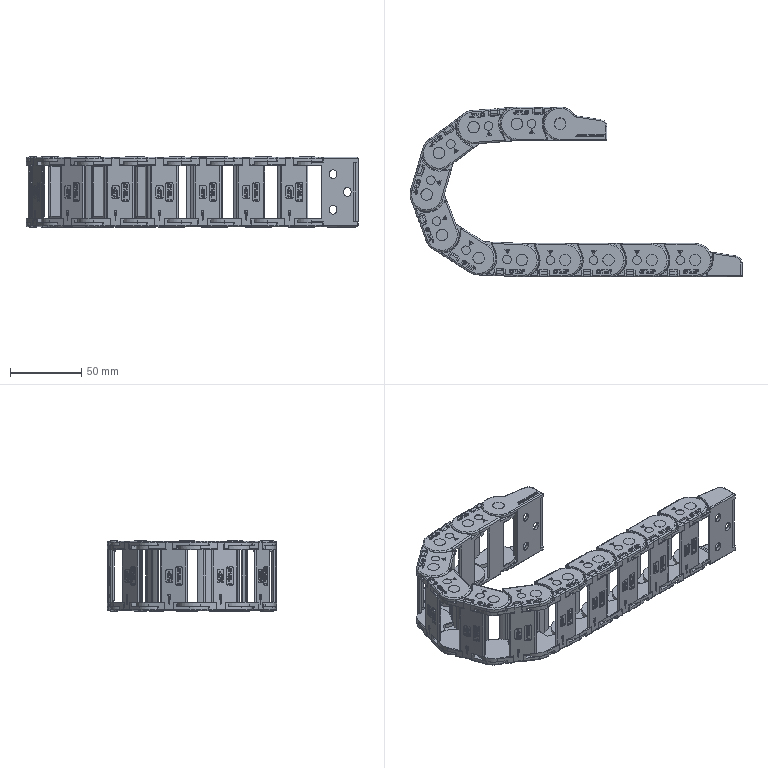Part | NX | features BREP 24 | 24 solids | 7167 faces | volume 130041 mm3 | plane 3923 | cylinder 1533 | spline 1456 | torus 231 | cone 24 | commonest cylinder face diameters 2 x299 1 x205 0.055 x132 23.5 x72 0.11 x66 8 x50